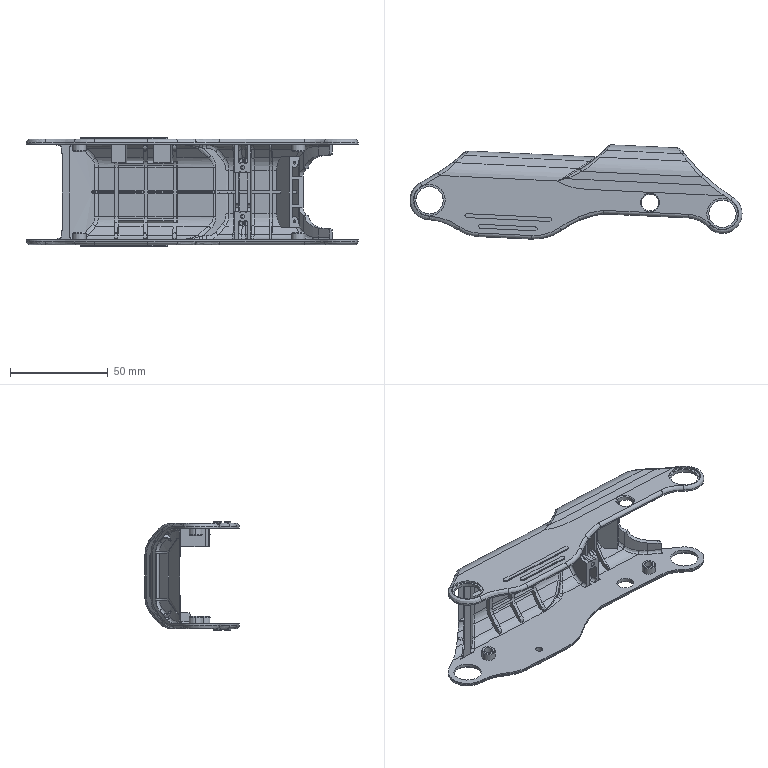Part | NX | features BREP 5, DATUM_CSYS 4, SKETCH 4, DELETE FACE 3, EXTRUDE 2 | 5 solids | 1010 faces | box 169.834 x 48.221 x 55.5 mm | volume 47491 mm3 | cylinder 412 | plane 294 | spline 151 | sphere 116 | torus 25 | cone 12 | commonest cylinder face diameters 1 x204 15 x24 20 x24 2.828 x14 14 x12 4 x11